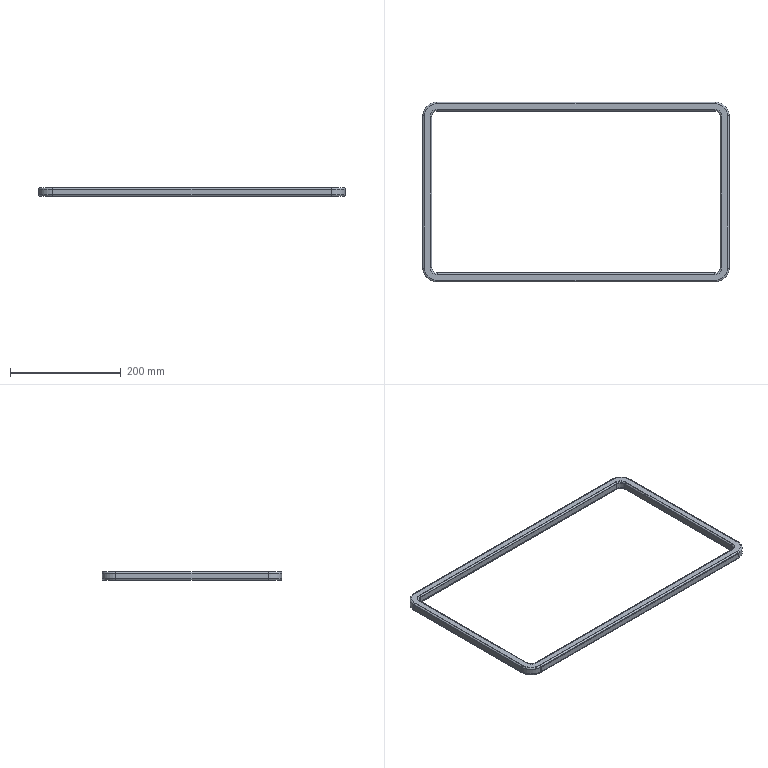Part | STEP file | 23.6 inch transparent screen outer fixing frame 001001 | 1 solid | 100 faces | box 554 x 325 x 16 mm | volume 92756 mm3 | cylinder 48 | torus 32 | plane 20 | commonest cylinder face diameters 4 x16 6 x16 20 x4 22 x4 48 x4 50 x4